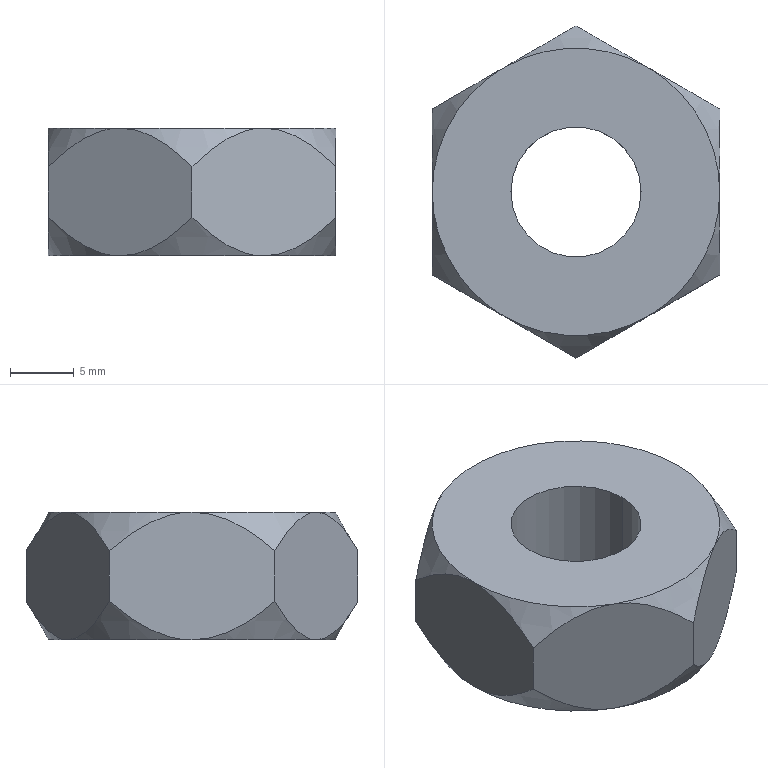Part | SolidWorks | features 3DProfileFeature 1, Extrusion 1, HoleWzd 1, ICE 1, MirrorPattern 1 | 1 solid | 22 faces | box 22.517 x 26 x 10 mm | volume 3499 mm3 | cone 12 | plane 8 | cylinder 2 | commonest cylinder face diameters 10.2 x2
STEP:
#1=CARTESIAN_POINT('',(-5.1,0.,-5.));
#2=VERTEX_POINT('',#1);
#3=CARTESIAN_POINT('',(5.1,0.,-5.));
#4=VERTEX_POINT('',#3);
#5=CARTESIAN_POINT('',(0.,0.,-5.));
#6=DIRECTION('',(0.,0.,1.));
#7=DIRECTION('',(1.,0.,0.));
#8=AXIS2_PLACEMENT_3D('',#5,#6,#7);
#9=CIRCLE('',#8,5.1);
#10=EDGE_CURVE('',#2,#4,#9,.T.);
#11=ORIENTED_EDGE('',*,*,#10,.F.);
#12=CARTESIAN_POINT('',(-5.1,0.,5.));
#13=VERTEX_POINT('',#12);
#14=CARTESIAN_POINT('',(-5.1,0.,5.));
#15=DIRECTION('',(0.,0.,1.));
#16=VECTOR('',#15,1000.);
#17=LINE('',#14,#16);
#18=EDGE_CURVE('',#2,#13,#17,.T.);
#19=ORIENTED_EDGE('',*,*,#18,.T.);
#20=CARTESIAN_POINT('',(5.1,0.,5.));
#21=VERTEX_POINT('',#20);
#22=CARTESIAN_POINT('',(0.,0.,5.));
#23=DIRECTION('',(0.,0.,1.));
#24=DIRECTION('',(1.,0.,0.));
#25=AXIS2_PLACEMENT_3D('',#22,#23,#24);
#26=CIRCLE('',#25,5.1);
#27=EDGE_CURVE('',#13,#21,#26,.T.);
#28=ORIENTED_EDGE('',*,*,#27,.T.);
#29=CARTESIAN_POINT('',(5.1,0.,5.));
#30=DIRECTION('',(0.,0.,1.));
#31=VECTOR('',#30,1000.);
#32=LINE('',#29,#31);
#33=EDGE_CURVE('',#4,#21,#32,.T.);
#34=ORIENTED_EDGE('',*,*,#33,.F.);
#35=EDGE_LOOP('',(#11,#19,#28,#34));
#36=FACE_OUTER_BOUND('',#35,.T.);
#37=CARTESIAN_POINT('',(0.,0.,5.));
#38=DIRECTION('',(0.,0.,1.));
#39=DIRECTION('',(1.,0.,0.));
#40=AXIS2_PLACEMENT_3D('',#37,#38,#39);
#41=CYLINDRICAL_SURFACE('',#40,5.1);
#42=ADVANCED_FACE('',(#36),#41,.F.);
#43=CARTESIAN_POINT('',(11.258,6.5,1.983));
#44=VERTEX_POINT('',#43);
#45=CARTESIAN_POINT('',(11.258,6.5,-1.983));
#46=VERTEX_POINT('',#45);
#47=CARTESIAN_POINT('',(11.258,6.5,5.));
#48=DIRECTION('',(0.,0.,-1.));
#49=VECTOR('',#48,1000.);
#50=LINE('',#47,#49);
#51=EDGE_CURVE('',#44,#46,#50,.T.);
#52=ORIENTED_EDGE('',*,*,#51,.T.);
#53=CARTESIAN_POINT('',(5.629,9.75,-5.));
#54=VERTEX_POINT('',#53);
#55=CARTESIAN_POINT('',(11.258,6.5,-1.983));
#56=CARTESIAN_POINT('',(10.858,6.731,-2.384));
#57=CARTESIAN_POINT('',(10.446,6.969,-2.764));
#58=CARTESIAN_POINT('',(9.589,7.464,-3.467));
#59=CARTESIAN_POINT('',(9.145,7.72,-3.79));
#60=CARTESIAN_POINT('',(8.441,8.126,-4.21));
#61=CARTESIAN_POINT('',(8.199,8.266,-4.34));
#62=CARTESIAN_POINT('',(7.705,8.551,-4.569));
#63=CARTESIAN_POINT('',(7.455,8.696,-4.667));
#64=CARTESIAN_POINT('',(6.946,8.99,-4.829));
#65=CARTESIAN_POINT('',(6.688,9.139,-4.892));
#66=CARTESIAN_POINT('',(6.162,9.442,-4.978));
#67=CARTESIAN_POINT('',(5.894,9.597,-5.));
#68=CARTESIAN_POINT('',(5.629,9.75,-5.));
#69=B_SPLINE_CURVE_WITH_KNOTS('',3,(#55,#56,#57,#58,#59,#60,#61,#62,#63,#64,#65,#66,#67,#68),.UNSPECIFIED.,.F.,.F.,(4,2,2,2,2,2,4),(0.000000303,0.001819,0.003638,0.004548,0.005458,0.006367,0.007277),.UNSPECIFIED.);
#70=EDGE_CURVE('',#46,#54,#69,.T.);
#71=ORIENTED_EDGE('',*,*,#70,.T.);
#72=CARTESIAN_POINT('',(0.,13.,-1.983));
#73=VERTEX_POINT('',#72);
#74=CARTESIAN_POINT('',(5.629,9.75,-5.));
#75=CARTESIAN_POINT('',(5.101,10.055,-5.));
#76=CARTESIAN_POINT('',(4.58,10.356,-4.914));
#77=CARTESIAN_POINT('',(3.553,10.949,-4.589));
#78=CARTESIAN_POINT('',(3.064,11.231,-4.356));
#79=CARTESIAN_POINT('',(2.129,11.771,-3.801));
#80=CARTESIAN_POINT('',(1.679,12.031,-3.475));
#81=CARTESIAN_POINT('',(0.8147,12.53,-2.766));
#82=CARTESIAN_POINT('',(0.401,12.768,-2.384));
#83=CARTESIAN_POINT('',(0.,13.,-1.983));
#84=B_SPLINE_CURVE_WITH_KNOTS('',3,(#74,#75,#76,#77,#78,#79,#80,#81,#82,#83),.UNSPECIFIED.,.F.,.F.,(4,2,2,2,4),(0.007277,0.009093,0.01091,0.01272,0.01454),.UNSPECIFIED.);
#85=EDGE_CURVE('',#54,#73,#84,.T.);
#86=ORIENTED_EDGE('',*,*,#85,.T.);
#87=CARTESIAN_POINT('',(0.,13.,1.983));
#88=VERTEX_POINT('',#87);
#89=CARTESIAN_POINT('',(0.,13.,5.));
#90=DIRECTION('',(0.,0.,-1.));
#91=VECTOR('',#90,1000.);
#92=LINE('',#89,#91);
#93=EDGE_CURVE('',#88,#73,#92,.T.);
#94=ORIENTED_EDGE('',*,*,#93,.F.);
#95=CARTESIAN_POINT('',(5.629,9.75,5.));
#96=VERTEX_POINT('',#95);
#97=CARTESIAN_POINT('',(5.629,9.75,5.));
#98=CARTESIAN_POINT('',(5.101,10.055,5.));
#99=CARTESIAN_POINT('',(4.58,10.356,4.914));
#100=CARTESIAN_POINT('',(3.553,10.949,4.589));
#101=CARTESIAN_POINT('',(3.064,11.231,4.356));
#102=CARTESIAN_POINT('',(2.129,11.771,3.801));
#103=CARTESIAN_POINT('',(1.679,12.031,3.475));
#104=CARTESIAN_POINT('',(0.8147,12.53,2.766));
#105=CARTESIAN_POINT('',(0.401,12.768,2.384));
#106=CARTESIAN_POINT('',(0.,13.,1.983));
#107=B_SPLINE_CURVE_WITH_KNOTS('',3,(#97,#98,#99,#100,#101,#102,#103,#104,#105,#106),.UNSPECIFIED.,.F.,.F.,(4,2,2,2,4),(0.007277,0.009093,0.01091,0.01272,0.01454),.UNSPECIFIED.);
#108=EDGE_CURVE('',#96,#88,#107,.T.);
#109=ORIENTED_EDGE('',*,*,#108,.F.);
#110=CARTESIAN_POINT('',(11.258,6.5,1.983));
#111=CARTESIAN_POINT('',(10.858,6.731,2.384));
#112=CARTESIAN_POINT('',(10.446,6.969,2.764));
#113=CARTESIAN_POINT('',(9.589,7.464,3.467));
#114=CARTESIAN_POINT('',(9.145,7.72,3.79));
#115=CARTESIAN_POINT('',(8.441,8.126,4.21));
#116=CARTESIAN_POINT('',(8.199,8.266,4.34));
#117=CARTESIAN_POINT('',(7.705,8.551,4.569));
#118=CARTESIAN_POINT('',(7.455,8.696,4.667));
#119=CARTESIAN_POINT('',(6.946,8.99,4.829));
#120=CARTESIAN_POINT('',(6.688,9.139,4.892));
#121=CARTESIAN_POINT('',(6.162,9.442,4.978));
#122=CARTESIAN_POINT('',(5.894,9.597,5.));
#123=CARTESIAN_POINT('',(5.629,9.75,5.));
#124=B_SPLINE_CURVE_WITH_KNOTS('',3,(#110,#111,#112,#113,#114,#115,#116,#117,#118,#119,#120,#121,#122,#123),.UNSPECIFIED.,.F.,.F.,(4,2,2,2,2,2,4),(0.000000303,0.001819,0.003638,0.004548,0.005458,0.006367,0.007277),.UNSPECIFIED.);
#125=EDGE_CURVE('',#44,#96,#124,.T.);
#126=ORIENTED_EDGE('',*,*,#125,.F.);
#127=EDGE_LOOP('',(#52,#71,#86,#94,#109,#126));
#128=FACE_OUTER_BOUND('',#127,.T.);
#129=CARTESIAN_POINT('',(11.258,6.5,5.));
#130=DIRECTION('',(-0.5,-0.866,0.));
#131=DIRECTION('',(0.866,-0.5,0.));
#132=AXIS2_PLACEMENT_3D('',#129,#130,#131);
#133=PLANE('',#132);
#134=ADVANCED_FACE('',(#128),#133,.F.);
#135=ORIENTED_EDGE('',*,*,#93,.T.);
#136=CARTESIAN_POINT('',(-5.629,9.75,-5.));
#137=VERTEX_POINT('',#136);
#138=CARTESIAN_POINT('',(0.,13.,-1.983));
#139=CARTESIAN_POINT('',(-0.4004,12.769,-2.384));
#140=CARTESIAN_POINT('',(-0.8123,12.531,-2.764));
#141=CARTESIAN_POINT('',(-1.669,12.036,-3.467));
#142=CARTESIAN_POINT('',(-2.113,11.78,-3.79));
#143=CARTESIAN_POINT('',(-2.817,11.374,-4.21));
#144=CARTESIAN_POINT('',(-3.059,11.234,-4.34));
#145=CARTESIAN_POINT('',(-3.553,10.949,-4.569));
#146=CARTESIAN_POINT('',(-3.803,10.804,-4.667));
#147=CARTESIAN_POINT('',(-4.312,10.51,-4.829));
#148=CARTESIAN_POINT('',(-4.57,10.361,-4.892));
#149=CARTESIAN_POINT('',(-5.096,10.058,-4.978));
#150=CARTESIAN_POINT('',(-5.365,9.903,-5.));
#151=CARTESIAN_POINT('',(-5.629,9.75,-5.));
#152=B_SPLINE_CURVE_WITH_KNOTS('',3,(#138,#139,#140,#141,#142,#143,#144,#145,#146,#147,#148,#149,#150,#151),.UNSPECIFIED.,.F.,.F.,(4,2,2,2,2,2,4),(0.000000303,0.001819,0.003638,0.004548,0.005458,0.006367,0.007277),.UNSPECIFIED.);
#153=EDGE_CURVE('',#73,#137,#152,.T.);
#154=ORIENTED_EDGE('',*,*,#153,.T.);
#155=CARTESIAN_POINT('',(-11.258,6.5,-1.983));
#156=VERTEX_POINT('',#155);
#157=CARTESIAN_POINT('',(-5.629,9.75,-5.));
#158=CARTESIAN_POINT('',(-6.157,9.445,-5.));
#159=CARTESIAN_POINT('',(-6.678,9.144,-4.914));
#160=CARTESIAN_POINT('',(-7.706,8.551,-4.589));
#161=CARTESIAN_POINT('',(-8.194,8.269,-4.356));
#162=CARTESIAN_POINT('',(-9.129,7.729,-3.801));
#163=CARTESIAN_POINT('',(-9.579,7.469,-3.475));
#164=CARTESIAN_POINT('',(-10.444,6.97,-2.766));
#165=CARTESIAN_POINT('',(-10.857,6.732,-2.384));
#166=CARTESIAN_POINT('',(-11.258,6.5,-1.983));
#167=B_SPLINE_CURVE_WITH_KNOTS('',3,(#157,#158,#159,#160,#161,#162,#163,#164,#165,#166),.UNSPECIFIED.,.F.,.F.,(4,2,2,2,4),(0.007277,0.009093,0.01091,0.01272,0.01454),.UNSPECIFIED.);
#168=EDGE_CURVE('',#137,#156,#167,.T.);
#169=ORIENTED_EDGE('',*,*,#168,.T.);
#170=CARTESIAN_POINT('',(-11.258,6.5,1.983));
#171=VERTEX_POINT('',#170);
#172=CARTESIAN_POINT('',(-11.258,6.5,5.));
#173=DIRECTION('',(0.,0.,-1.));
#174=VECTOR('',#173,1000.);
#175=LINE('',#172,#174);
#176=EDGE_CURVE('',#171,#156,#175,.T.);
#177=ORIENTED_EDGE('',*,*,#176,.F.);
#178=CARTESIAN_POINT('',(-5.629,9.75,5.));
#179=VERTEX_POINT('',#178);
#180=CARTESIAN_POINT('',(-5.629,9.75,5.));
#181=CARTESIAN_POINT('',(-6.157,9.445,5.));
#182=CARTESIAN_POINT('',(-6.678,9.144,4.914));
#183=CARTESIAN_POINT('',(-7.706,8.551,4.589));
#184=CARTESIAN_POINT('',(-8.194,8.269,4.356));
#185=CARTESIAN_POINT('',(-9.129,7.729,3.801));
#186=CARTESIAN_POINT('',(-9.579,7.469,3.475));
#187=CARTESIAN_POINT('',(-10.444,6.97,2.766));
#188=CARTESIAN_POINT('',(-10.857,6.732,2.384));
#189=CARTESIAN_POINT('',(-11.258,6.5,1.983));
#190=B_SPLINE_CURVE_WITH_KNOTS('',3,(#180,#181,#182,#183,#184,#185,#186,#187,#188,#189),.UNSPECIFIED.,.F.,.F.,(4,2,2,2,4),(0.007277,0.009093,0.01091,0.01272,0.01454),.UNSPECIFIED.);
#191=EDGE_CURVE('',#179,#171,#190,.T.);
#192=ORIENTED_EDGE('',*,*,#191,.F.);
#193=CARTESIAN_POINT('',(0.,13.,1.983));
#194=CARTESIAN_POINT('',(-0.4004,12.769,2.384));
#195=CARTESIAN_POINT('',(-0.8123,12.531,2.764));
#196=CARTESIAN_POINT('',(-1.669,12.036,3.467));
#197=CARTESIAN_POINT('',(-2.113,11.78,3.79));
#198=CARTESIAN_POINT('',(-2.817,11.374,4.21));
#199=CARTESIAN_POINT('',(-3.059,11.234,4.34));
#200=CARTESIAN_POINT('',(-3.553,10.949,4.569));
#201=CARTESIAN_POINT('',(-3.803,10.804,4.667));
#202=CARTESIAN_POINT('',(-4.312,10.51,4.829));
#203=CARTESIAN_POINT('',(-4.57,10.361,4.892));
#204=CARTESIAN_POINT('',(-5.096,10.058,4.978));
#205=CARTESIAN_POINT('',(-5.365,9.903,5.));
#206=CARTESIAN_POINT('',(-5.629,9.75,5.));
#207=B_SPLINE_CURVE_WITH_KNOTS('',3,(#193,#194,#195,#196,#197,#198,#199,#200,#201,#202,#203,#204,#205,#206),.UNSPECIFIED.,.F.,.F.,(4,2,2,2,2,2,4),(0.000000303,0.001819,0.003638,0.004548,0.005458,0.006367,0.007277),.UNSPECIFIED.);
#208=EDGE_CURVE('',#88,#179,#207,.T.);
#209=ORIENTED_EDGE('',*,*,#208,.F.);
#210=EDGE_LOOP('',(#135,#154,#169,#177,#192,#209));
#211=FACE_OUTER_BOUND('',#210,.T.);
#212=CARTESIAN_POINT('',(0.,13.,5.));
#213=DIRECTION('',(0.5,-0.866,0.));
#214=DIRECTION('',(0.866,0.5,0.));
#215=AXIS2_PLACEMENT_3D('',#212,#213,#214);
#216=PLANE('',#215);
#217=ADVANCED_FACE('',(#211),#216,.F.);
#218=ORIENTED_EDGE('',*,*,#176,.T.);
#219=CARTESIAN_POINT('',(-11.258,0.,-5.));
#220=VERTEX_POINT('',#219);
#221=CARTESIAN_POINT('',(-11.258,6.5,-1.983));
#222=CARTESIAN_POINT('',(-11.258,6.271,-2.182));
#223=CARTESIAN_POINT('',(-11.258,6.038,-2.376));
#224=CARTESIAN_POINT('',(-11.258,5.56,-2.755));
#225=CARTESIAN_POINT('',(-11.258,5.315,-2.94));
#226=CARTESIAN_POINT('',(-11.258,4.568,-3.471));
#227=CARTESIAN_POINT('',(-11.258,4.053,-3.794));
#228=CARTESIAN_POINT('',(-11.258,3.243,-4.212));
#229=CARTESIAN_POINT('',(-11.258,2.966,-4.34));
#230=CARTESIAN_POINT('',(-11.258,2.398,-4.568));
#231=CARTESIAN_POINT('',(-11.258,2.105,-4.668));
#232=CARTESIAN_POINT('',(-11.258,1.516,-4.83));
#233=CARTESIAN_POINT('',(-11.258,1.218,-4.893));
#234=CARTESIAN_POINT('',(-11.258,0.6148,-4.978));
#235=CARTESIAN_POINT('',(-11.258,0.3082,-5.));
#236=CARTESIAN_POINT('',(-11.258,0.,-5.));
#237=B_SPLINE_CURVE_WITH_KNOTS('',3,(#221,#222,#223,#224,#225,#226,#227,#228,#229,#230,#231,#232,#233,#234,#235,#236),.UNSPECIFIED.,.F.,.F.,(4,2,2,2,2,2,2,4),(0.01214,0.01304,0.01394,0.01574,0.01665,0.01755,0.01845,0.01935),.UNSPECIFIED.);
#238=EDGE_CURVE('',#156,#220,#237,.T.);
#239=ORIENTED_EDGE('',*,*,#238,.T.);
#240=CARTESIAN_POINT('',(-11.258,-6.5,-1.983));
#241=VERTEX_POINT('',#240);
#242=CARTESIAN_POINT('',(-11.258,0.,-5.));
#243=CARTESIAN_POINT('',(-11.258,-0.6167,-5.));
#244=CARTESIAN_POINT('',(-11.258,-1.219,-4.912));
#245=CARTESIAN_POINT('',(-11.258,-2.105,-4.668));
#246=CARTESIAN_POINT('',(-11.258,-2.398,-4.568));
#247=CARTESIAN_POINT('',(-11.258,-2.966,-4.341));
#248=CARTESIAN_POINT('',(-11.258,-3.242,-4.213));
#249=CARTESIAN_POINT('',(-11.258,-4.052,-3.795));
#250=CARTESIAN_POINT('',(-11.258,-4.567,-3.471));
#251=CARTESIAN_POINT('',(-11.258,-5.565,-2.762));
#252=CARTESIAN_POINT('',(-11.258,-6.042,-2.38));
#253=CARTESIAN_POINT('',(-11.258,-6.5,-1.983));
#254=B_SPLINE_CURVE_WITH_KNOTS('',3,(#242,#243,#244,#245,#246,#247,#248,#249,#250,#251,#252,#253),.UNSPECIFIED.,.F.,.F.,(4,2,2,2,2,4),(0.01935,0.02115,0.02206,0.02296,0.02476,0.02656),.UNSPECIFIED.);
#255=EDGE_CURVE('',#220,#241,#254,.T.);
#256=ORIENTED_EDGE('',*,*,#255,.T.);
#257=CARTESIAN_POINT('',(-11.258,-6.5,1.983));
#258=VERTEX_POINT('',#257);
#259=CARTESIAN_POINT('',(-11.258,-6.5,5.));
#260=DIRECTION('',(0.,0.,-1.));
#261=VECTOR('',#260,1000.);
#262=LINE('',#259,#261);
#263=EDGE_CURVE('',#258,#241,#262,.T.);
#264=ORIENTED_EDGE('',*,*,#263,.F.);
#265=CARTESIAN_POINT('',(-11.258,0.,5.));
#266=VERTEX_POINT('',#265);
#267=CARTESIAN_POINT('',(-11.258,0.,5.));
#268=CARTESIAN_POINT('',(-11.258,-0.6167,5.));
#269=CARTESIAN_POINT('',(-11.258,-1.219,4.912));
#270=CARTESIAN_POINT('',(-11.258,-2.105,4.668));
#271=CARTESIAN_POINT('',(-11.258,-2.398,4.568));
#272=CARTESIAN_POINT('',(-11.258,-2.966,4.341));
#273=CARTESIAN_POINT('',(-11.258,-3.242,4.213));
#274=CARTESIAN_POINT('',(-11.258,-4.052,3.795));
#275=CARTESIAN_POINT('',(-11.258,-4.567,3.471));
#276=CARTESIAN_POINT('',(-11.258,-5.565,2.762));
#277=CARTESIAN_POINT('',(-11.258,-6.042,2.38));
#278=CARTESIAN_POINT('',(-11.258,-6.5,1.983));
#279=B_SPLINE_CURVE_WITH_KNOTS('',3,(#267,#268,#269,#270,#271,#272,#273,#274,#275,#276,#277,#278),.UNSPECIFIED.,.F.,.F.,(4,2,2,2,2,4),(0.01935,0.02115,0.02206,0.02296,0.02476,0.02656),.UNSPECIFIED.);
#280=EDGE_CURVE('',#266,#258,#279,.T.);
#281=ORIENTED_EDGE('',*,*,#280,.F.);
#282=CARTESIAN_POINT('',(-11.258,6.5,1.983));
#283=CARTESIAN_POINT('',(-11.258,6.271,2.182));
#284=CARTESIAN_POINT('',(-11.258,6.038,2.376));
#285=CARTESIAN_POINT('',(-11.258,5.56,2.755));
#286=CARTESIAN_POINT('',(-11.258,5.315,2.94));
#287=CARTESIAN_POINT('',(-11.258,4.568,3.471));
#288=CARTESIAN_POINT('',(-11.258,4.053,3.794));
#289=CARTESIAN_POINT('',(-11.258,3.243,4.212));
#290=CARTESIAN_POINT('',(-11.258,2.966,4.34));
#291=CARTESIAN_POINT('',(-11.258,2.398,4.568));
#292=CARTESIAN_POINT('',(-11.258,2.105,4.668));
#293=CARTESIAN_POINT('',(-11.258,1.516,4.83));
#294=CARTESIAN_POINT('',(-11.258,1.218,4.893));
#295=CARTESIAN_POINT('',(-11.258,0.6148,4.978));
#296=CARTESIAN_POINT('',(-11.258,0.3082,5.));
#297=CARTESIAN_POINT('',(-11.258,0.,5.));
#298=B_SPLINE_CURVE_WITH_KNOTS('',3,(#282,#283,#284,#285,#286,#287,#288,#289,#290,#291,#292,#293,#294,#295,#296,#297),.UNSPECIFIED.,.F.,.F.,(4,2,2,2,2,2,2,4),(0.01214,0.01304,0.01394,0.01574,0.01665,0.01755,0.01845,0.01935),.UNSPECIFIED.);
#299=EDGE_CURVE('',#171,#266,#298,.T.);
#300=ORIENTED_EDGE('',*,*,#299,.F.);
#301=EDGE_LOOP('',(#218,#239,#256,#264,#281,#300));
#302=FACE_OUTER_BOUND('',#301,.T.);
#303=CARTESIAN_POINT('',(-11.258,6.5,5.));
#304=DIRECTION('',(1.,0.,0.));
#305=DIRECTION('',(0.,0.,-1.));
#306=AXIS2_PLACEMENT_3D('',#303,#304,#305);
#307=PLANE('',#306);
#308=ADVANCED_FACE('',(#302),#307,.F.);
#309=ORIENTED_EDGE('',*,*,#263,.T.);
#310=CARTESIAN_POINT('',(-5.629,-9.75,-5.));
#311=VERTEX_POINT('',#310);
#312=CARTESIAN_POINT('',(-11.258,-6.5,-1.983));
#313=CARTESIAN_POINT('',(-10.858,-6.731,-2.384));
#314=CARTESIAN_POINT('',(-10.446,-6.969,-2.764));
#315=CARTESIAN_POINT('',(-9.589,-7.464,-3.467));
#316=CARTESIAN_POINT('',(-9.145,-7.72,-3.79));
#317=CARTESIAN_POINT('',(-8.441,-8.126,-4.21));
#318=CARTESIAN_POINT('',(-8.199,-8.266,-4.34));
#319=CARTESIAN_POINT('',(-7.705,-8.551,-4.569));
#320=CARTESIAN_POINT('',(-7.455,-8.696,-4.667));
#321=CARTESIAN_POINT('',(-6.946,-8.99,-4.829));
#322=CARTESIAN_POINT('',(-6.688,-9.139,-4.892));
#323=CARTESIAN_POINT('',(-6.162,-9.442,-4.978));
#324=CARTESIAN_POINT('',(-5.894,-9.597,-5.));
#325=CARTESIAN_POINT('',(-5.629,-9.75,-5.));
#326=B_SPLINE_CURVE_WITH_KNOTS('',3,(#312,#313,#314,#315,#316,#317,#318,#319,#320,#321,#322,#323,#324,#325),.UNSPECIFIED.,.F.,.F.,(4,2,2,2,2,2,4),(0.000000303,0.001819,0.003638,0.004548,0.005458,0.006367,0.007277),.UNSPECIFIED.);
#327=EDGE_CURVE('',#241,#311,#326,.T.);
#328=ORIENTED_EDGE('',*,*,#327,.T.);
#329=CARTESIAN_POINT('',(0.,-13.,-1.983));
#330=VERTEX_POINT('',#329);
#331=CARTESIAN_POINT('',(-5.629,-9.75,-5.));
#332=CARTESIAN_POINT('',(-5.101,-10.055,-5.));
#333=CARTESIAN_POINT('',(-4.58,-10.356,-4.914));
#334=CARTESIAN_POINT('',(-3.553,-10.949,-4.589));
#335=CARTESIAN_POINT('',(-3.064,-11.231,-4.356));
#336=CARTESIAN_POINT('',(-2.129,-11.771,-3.801));
#337=CARTESIAN_POINT('',(-1.679,-12.031,-3.475));
#338=CARTESIAN_POINT('',(-0.8147,-12.53,-2.766));
#339=CARTESIAN_POINT('',(-0.401,-12.768,-2.384));
#340=CARTESIAN_POINT('',(0.,-13.,-1.983));
#341=B_SPLINE_CURVE_WITH_KNOTS('',3,(#331,#332,#333,#334,#335,#336,#337,#338,#339,#340),.UNSPECIFIED.,.F.,.F.,(4,2,2,2,4),(0.007277,0.009093,0.01091,0.01272,0.01454),.UNSPECIFIED.);
#342=EDGE_CURVE('',#311,#330,#341,.T.);
#343=ORIENTED_EDGE('',*,*,#342,.T.);
#344=CARTESIAN_POINT('',(0.,-13.,1.983));
#345=VERTEX_POINT('',#344);
#346=CARTESIAN_POINT('',(0.,-13.,5.));
#347=DIRECTION('',(0.,0.,-1.));
#348=VECTOR('',#347,1000.);
#349=LINE('',#346,#348);
#350=EDGE_CURVE('',#345,#330,#349,.T.);
#351=ORIENTED_EDGE('',*,*,#350,.F.);
#352=CARTESIAN_POINT('',(-5.629,-9.75,5.));
#353=VERTEX_POINT('',#352);
#354=CARTESIAN_POINT('',(-5.629,-9.75,5.));
#355=CARTESIAN_POINT('',(-5.101,-10.055,5.));
#356=CARTESIAN_POINT('',(-4.58,-10.356,4.914));
#357=CARTESIAN_POINT('',(-3.553,-10.949,4.589));
#358=CARTESIAN_POINT('',(-3.064,-11.231,4.356));
#359=CARTESIAN_POINT('',(-2.129,-11.771,3.801));
#360=CARTESIAN_POINT('',(-1.679,-12.031,3.475));
#361=CARTESIAN_POINT('',(-0.8147,-12.53,2.766));
#362=CARTESIAN_POINT('',(-0.401,-12.768,2.384));
#363=CARTESIAN_POINT('',(0.,-13.,1.983));
#364=B_SPLINE_CURVE_WITH_KNOTS('',3,(#354,#355,#356,#357,#358,#359,#360,#361,#362,#363),.UNSPECIFIED.,.F.,.F.,(4,2,2,2,4),(0.007277,0.009093,0.01091,0.01272,0.01454),.UNSPECIFIED.);
#365=EDGE_CURVE('',#353,#345,#364,.T.);
#366=ORIENTED_EDGE('',*,*,#365,.F.);
#367=CARTESIAN_POINT('',(-11.258,-6.5,1.983));
#368=CARTESIAN_POINT('',(-10.858,-6.731,2.384));
#369=CARTESIAN_POINT('',(-10.446,-6.969,2.764));
#370=CARTESIAN_POINT('',(-9.589,-7.464,3.467));
#371=CARTESIAN_POINT('',(-9.145,-7.72,3.79));
#372=CARTESIAN_POINT('',(-8.441,-8.126,4.21));
#373=CARTESIAN_POINT('',(-8.199,-8.266,4.34));
#374=CARTESIAN_POINT('',(-7.705,-8.551,4.569));
#375=CARTESIAN_POINT('',(-7.455,-8.696,4.667));
#376=CARTESIAN_POINT('',(-6.946,-8.99,4.829));
#377=CARTESIAN_POINT('',(-6.688,-9.139,4.892));
#378=CARTESIAN_POINT('',(-6.162,-9.442,4.978));
#379=CARTESIAN_POINT('',(-5.894,-9.597,5.));
#380=CARTESIAN_POINT('',(-5.629,-9.75,5.));
#381=B_SPLINE_CURVE_WITH_KNOTS('',3,(#367,#368,#369,#370,#371,#372,#373,#374,#375,#376,#377,#378,#379,#380),.UNSPECIFIED.,.F.,.F.,(4,2,2,2,2,2,4),(0.000000303,0.001819,0.003638,0.004548,0.005458,0.006367,0.007277),.UNSPECIFIED.);
#382=EDGE_CURVE('',#258,#353,#381,.T.);
#383=ORIENTED_EDGE('',*,*,#382,.F.);
#384=EDGE_LOOP('',(#309,#328,#343,#351,#366,#383));
#385=FACE_OUTER_BOUND('',#384,.T.);
#386=CARTESIAN_POINT('',(-11.258,-6.5,5.));
#387=DIRECTION('',(0.5,0.866,0.));
#388=DIRECTION('',(-0.866,0.5,0.));
#389=AXIS2_PLACEMENT_3D('',#386,#387,#388);
#390=PLANE('',#389);
#391=ADVANCED_FACE('',(#385),#390,.F.);
#392=ORIENTED_EDGE('',*,*,#350,.T.);
#393=CARTESIAN_POINT('',(5.629,-9.75,-5.));
#394=VERTEX_POINT('',#393);
#395=CARTESIAN_POINT('',(0.,-13.,-1.983));
#396=CARTESIAN_POINT('',(0.4004,-12.769,-2.384));
#397=CARTESIAN_POINT('',(0.8123,-12.531,-2.764));
#398=CARTESIAN_POINT('',(1.669,-12.036,-3.467));
#399=CARTESIAN_POINT('',(2.113,-11.78,-3.79));
#400=CARTESIAN_POINT('',(2.817,-11.374,-4.21));
#401=CARTESIAN_POINT('',(3.059,-11.234,-4.34));
#402=CARTESIAN_POINT('',(3.553,-10.949,-4.569));
#403=CARTESIAN_POINT('',(3.803,-10.804,-4.667));
#404=CARTESIAN_POINT('',(4.312,-10.51,-4.829));
#405=CARTESIAN_POINT('',(4.57,-10.361,-4.892));
#406=CARTESIAN_POINT('',(5.096,-10.058,-4.978));
#407=CARTESIAN_POINT('',(5.365,-9.903,-5.));
#408=CARTESIAN_POINT('',(5.629,-9.75,-5.));
#409=B_SPLINE_CURVE_WITH_KNOTS('',3,(#395,#396,#397,#398,#399,#400,#401,#402,#403,#404,#405,#406,#407,#408),.UNSPECIFIED.,.F.,.F.,(4,2,2,2,2,2,4),(0.000000303,0.001819,0.003638,0.004548,0.005458,0.006367,0.007277),.UNSPECIFIED.);
#410=EDGE_CURVE('',#330,#394,#409,.T.);
#411=ORIENTED_EDGE('',*,*,#410,.T.);
#412=CARTESIAN_POINT('',(11.258,-6.5,-1.983));
#413=VERTEX_POINT('',#412);
#414=CARTESIAN_POINT('',(5.629,-9.75,-5.));
#415=CARTESIAN_POINT('',(6.157,-9.445,-5.));
#416=CARTESIAN_POINT('',(6.678,-9.144,-4.914));
#417=CARTESIAN_POINT('',(7.706,-8.551,-4.589));
#418=CARTESIAN_POINT('',(8.194,-8.269,-4.356));
#419=CARTESIAN_POINT('',(9.129,-7.729,-3.801));
#420=CARTESIAN_POINT('',(9.579,-7.469,-3.475));
#421=CARTESIAN_POINT('',(10.444,-6.97,-2.766));
#422=CARTESIAN_POINT('',(10.857,-6.732,-2.384));
#423=CARTESIAN_POINT('',(11.258,-6.5,-1.983));
#424=B_SPLINE_CURVE_WITH_KNOTS('',3,(#414,#415,#416,#417,#418,#419,#420,#421,#422,#423),.UNSPECIFIED.,.F.,.F.,(4,2,2,2,4),(0.007277,0.009093,0.01091,0.01272,0.01454),.UNSPECIFIED.);
#425=EDGE_CURVE('',#394,#413,#424,.T.);
#426=ORIENTED_EDGE('',*,*,#425,.T.);
#427=CARTESIAN_POINT('',(11.258,-6.5,1.983));
#428=VERTEX_POINT('',#427);
#429=CARTESIAN_POINT('',(11.258,-6.5,5.));
#430=DIRECTION('',(0.,0.,-1.));
#431=VECTOR('',#430,1000.);
#432=LINE('',#429,#431);
#433=EDGE_CURVE('',#428,#413,#432,.T.);
#434=ORIENTED_EDGE('',*,*,#433,.F.);
#435=CARTESIAN_POINT('',(5.629,-9.75,5.));
#436=VERTEX_POINT('',#435);
#437=CARTESIAN_POINT('',(5.629,-9.75,5.));
#438=CARTESIAN_POINT('',(6.157,-9.445,5.));
#439=CARTESIAN_POINT('',(6.678,-9.144,4.914));
#440=CARTESIAN_POINT('',(7.706,-8.551,4.589));
#441=CARTESIAN_POINT('',(8.194,-8.269,4.356));
#442=CARTESIAN_POINT('',(9.129,-7.729,3.801));
#443=CARTESIAN_POINT('',(9.579,-7.469,3.475));
#444=CARTESIAN_POINT('',(10.444,-6.97,2.766));
#445=CARTESIAN_POINT('',(10.857,-6.732,2.384));
#446=CARTESIAN_POINT('',(11.258,-6.5,1.983));
#447=B_SPLINE_CURVE_WITH_KNOTS('',3,(#437,#438,#439,#440,#441,#442,#443,#444,#445,#446),.UNSPECIFIED.,.F.,.F.,(4,2,2,2,4),(0.007277,0.009093,0.01091,0.01272,0.01454),.UNSPECIFIED.);
#448=EDGE_CURVE('',#436,#428,#447,.T.);
#449=ORIENTED_EDGE('',*,*,#448,.F.);
#450=CARTESIAN_POINT('',(0.,-13.,1.983));
#451=CARTESIAN_POINT('',(0.4004,-12.769,2.384));
#452=CARTESIAN_POINT('',(0.8123,-12.531,2.764));
#453=CARTESIAN_POINT('',(1.669,-12.036,3.467));
#454=CARTESIAN_POINT('',(2.113,-11.78,3.79));
#455=CARTESIAN_POINT('',(2.817,-11.374,4.21));
#456=CARTESIAN_POINT('',(3.059,-11.234,4.34));
#457=CARTESIAN_POINT('',(3.553,-10.949,4.569));
#458=CARTESIAN_POINT('',(3.803,-10.804,4.667));
#459=CARTESIAN_POINT('',(4.312,-10.51,4.829));
#460=CARTESIAN_POINT('',(4.57,-10.361,4.892));
#461=CARTESIAN_POINT('',(5.096,-10.058,4.978));
#462=CARTESIAN_POINT('',(5.365,-9.903,5.));
#463=CARTESIAN_POINT('',(5.629,-9.75,5.));
#464=B_SPLINE_CURVE_WITH_KNOTS('',3,(#450,#451,#452,#453,#454,#455,#456,#457,#458,#459,#460,#461,#462,#463),.UNSPECIFIED.,.F.,.F.,(4,2,2,2,2,2,4),(0.000000303,0.001819,0.003638,0.004548,0.005458,0.006367,0.007277),.UNSPECIFIED.);
#465=EDGE_CURVE('',#345,#436,#464,.T.);
#466=ORIENTED_EDGE('',*,*,#465,.F.);
#467=EDGE_LOOP('',(#392,#411,#426,#434,#449,#466));
#468=FACE_OUTER_BOUND('',#467,.T.);
#469=CARTESIAN_POINT('',(0.,-13.,5.));
#470=DIRECTION('',(-0.5,0.866,0.));
#471=DIRECTION('',(-0.866,-0.5,0.));
#472=AXIS2_PLACEMENT_3D('',#469,#470,#471);
#473=PLANE('',#472);
#474=ADVANCED_FACE('',(#468),#473,.F.);
#475=ORIENTED_EDGE('',*,*,#433,.T.);
#476=CARTESIAN_POINT('',(11.258,0.,-5.));
#477=VERTEX_POINT('',#476);
#478=CARTESIAN_POINT('',(11.258,-6.5,-1.983));
#479=CARTESIAN_POINT('',(11.258,-6.042,-2.38));
#480=CARTESIAN_POINT('',(11.258,-5.565,-2.762));
#481=CARTESIAN_POINT('',(11.258,-4.567,-3.471));
#482=CARTESIAN_POINT('',(11.258,-4.052,-3.795));
#483=CARTESIAN_POINT('',(11.258,-3.242,-4.213));
#484=CARTESIAN_POINT('',(11.258,-2.966,-4.341));
#485=CARTESIAN_POINT('',(11.258,-2.398,-4.568));
#486=CARTESIAN_POINT('',(11.258,-2.105,-4.668));
#487=CARTESIAN_POINT('',(11.258,-1.219,-4.912));
#488=CARTESIAN_POINT('',(11.258,-0.6167,-5.));
#489=CARTESIAN_POINT('',(11.258,0.,-5.));
#490=B_SPLINE_CURVE_WITH_KNOTS('',3,(#478,#479,#480,#481,#482,#483,#484,#485,#486,#487,#488,#489),.UNSPECIFIED.,.F.,.F.,(4,2,2,2,2,4),(0.00934,0.01115,0.01296,0.01386,0.01477,0.01657),.UNSPECIFIED.);
#491=EDGE_CURVE('',#413,#477,#490,.T.);
#492=ORIENTED_EDGE('',*,*,#491,.T.);
#493=CARTESIAN_POINT('',(11.258,0.,-5.));
#494=CARTESIAN_POINT('',(11.258,0.3082,-5.));
#495=CARTESIAN_POINT('',(11.258,0.6148,-4.978));
#496=CARTESIAN_POINT('',(11.258,1.218,-4.893));
#497=CARTESIAN_POINT('',(11.258,1.516,-4.83));
#498=CARTESIAN_POINT('',(11.258,2.105,-4.668));
#499=CARTESIAN_POINT('',(11.258,2.398,-4.568));
#500=CARTESIAN_POINT('',(11.258,2.966,-4.34));
#501=CARTESIAN_POINT('',(11.258,3.243,-4.212));
#502=CARTESIAN_POINT('',(11.258,4.053,-3.794));
#503=CARTESIAN_POINT('',(11.258,4.568,-3.471));
#504=CARTESIAN_POINT('',(11.258,5.315,-2.94));
#505=CARTESIAN_POINT('',(11.258,5.56,-2.755));
#506=CARTESIAN_POINT('',(11.258,6.038,-2.376));
#507=CARTESIAN_POINT('',(11.258,6.271,-2.182));
#508=CARTESIAN_POINT('',(11.258,6.5,-1.983));
#509=B_SPLINE_CURVE_WITH_KNOTS('',3,(#493,#494,#495,#496,#497,#498,#499,#500,#501,#502,#503,#504,#505,#506,#507,#508),.UNSPECIFIED.,.F.,.F.,(4,2,2,2,2,2,2,4),(0.01657,0.01748,0.01838,0.01929,0.02019,0.022,0.0229,0.0238),.UNSPECIFIED.);
#510=EDGE_CURVE('',#477,#46,#509,.T.);
#511=ORIENTED_EDGE('',*,*,#510,.T.);
#512=ORIENTED_EDGE('',*,*,#51,.F.);
#513=CARTESIAN_POINT('',(11.258,0.,5.));
#514=VERTEX_POINT('',#513);
#515=CARTESIAN_POINT('',(11.258,0.,5.));
#516=CARTESIAN_POINT('',(11.258,0.3082,5.));
#517=CARTESIAN_POINT('',(11.258,0.6148,4.978));
#518=CARTESIAN_POINT('',(11.258,1.218,4.893));
#519=CARTESIAN_POINT('',(11.258,1.516,4.83));
#520=CARTESIAN_POINT('',(11.258,2.105,4.668));
#521=CARTESIAN_POINT('',(11.258,2.398,4.568));
#522=CARTESIAN_POINT('',(11.258,2.966,4.34));
#523=CARTESIAN_POINT('',(11.258,3.243,4.212));
#524=CARTESIAN_POINT('',(11.258,4.053,3.794));
#525=CARTESIAN_POINT('',(11.258,4.568,3.471));
#526=CARTESIAN_POINT('',(11.258,5.315,2.94));
#527=CARTESIAN_POINT('',(11.258,5.56,2.755));
#528=CARTESIAN_POINT('',(11.258,6.038,2.376));
#529=CARTESIAN_POINT('',(11.258,6.271,2.182));
#530=CARTESIAN_POINT('',(11.258,6.5,1.983));
#531=B_SPLINE_CURVE_WITH_KNOTS('',3,(#515,#516,#517,#518,#519,#520,#521,#522,#523,#524,#525,#526,#527,#528,#529,#530),.UNSPECIFIED.,.F.,.F.,(4,2,2,2,2,2,2,4),(0.01657,0.01748,0.01838,0.01929,0.02019,0.022,0.0229,0.0238),.UNSPECIFIED.);
#532=EDGE_CURVE('',#514,#44,#531,.T.);
#533=ORIENTED_EDGE('',*,*,#532,.F.);
#534=CARTESIAN_POINT('',(11.258,-6.5,1.983));
#535=CARTESIAN_POINT('',(11.258,-6.042,2.38));
#536=CARTESIAN_POINT('',(11.258,-5.565,2.762));
#537=CARTESIAN_POINT('',(11.258,-4.567,3.471));
#538=CARTESIAN_POINT('',(11.258,-4.052,3.795));
#539=CARTESIAN_POINT('',(11.258,-3.242,4.213));
#540=CARTESIAN_POINT('',(11.258,-2.966,4.341));
#541=CARTESIAN_POINT('',(11.258,-2.398,4.568));
#542=CARTESIAN_POINT('',(11.258,-2.105,4.668));
#543=CARTESIAN_POINT('',(11.258,-1.219,4.912));
#544=CARTESIAN_POINT('',(11.258,-0.6167,5.));
#545=CARTESIAN_POINT('',(11.258,0.,5.));
#546=B_SPLINE_CURVE_WITH_KNOTS('',3,(#534,#535,#536,#537,#538,#539,#540,#541,#542,#543,#544,#545),.UNSPECIFIED.,.F.,.F.,(4,2,2,2,2,4),(0.00934,0.01115,0.01296,0.01386,0.01477,0.01657),.UNSPECIFIED.);
#547=EDGE_CURVE('',#428,#514,#546,.T.);
#548=ORIENTED_EDGE('',*,*,#547,.F.);
#549=EDGE_LOOP('',(#475,#492,#511,#512,#533,#548));
#550=FACE_OUTER_BOUND('',#549,.T.);
#551=CARTESIAN_POINT('',(11.258,-6.5,5.));
#552=DIRECTION('',(-1.,0.,0.));
#553=DIRECTION('',(0.,-1.,0.));
#554=AXIS2_PLACEMENT_3D('',#551,#552,#553);
#555=PLANE('',#554);
#556=ADVANCED_FACE('',(#550),#555,.F.);
#557=ORIENTED_EDGE('',*,*,#448,.T.);
#558=ORIENTED_EDGE('',*,*,#547,.T.);
#559=CARTESIAN_POINT('',(0.,0.,5.));
#560=DIRECTION('',(0.,0.,1.));
#561=DIRECTION('',(1.,0.,0.));
#562=AXIS2_PLACEMENT_3D('',#559,#560,#561);
#563=CIRCLE('',#562,11.258);
#564=EDGE_CURVE('',#436,#514,#563,.T.);
#565=ORIENTED_EDGE('',*,*,#564,.F.);
#566=EDGE_LOOP('',(#557,#558,#565));
#567=FACE_OUTER_BOUND('',#566,.T.);
#568=CARTESIAN_POINT('',(0.,0.,5.));
#569=DIRECTION('',(0.,0.,-1.));
#570=DIRECTION('',(1.,0.,0.));
#571=AXIS2_PLACEMENT_3D('',#568,#569,#570);
#572=CONICAL_SURFACE('',#571,11.258,0.5236);
#573=ADVANCED_FACE('',(#567),#572,.T.);
#574=ORIENTED_EDGE('',*,*,#365,.T.);
#575=ORIENTED_EDGE('',*,*,#465,.T.);
#576=CARTESIAN_POINT('',(0.,0.,5.));
#577=DIRECTION('',(0.,0.,1.));
#578=DIRECTION('',(1.,0.,0.));
#579=AXIS2_PLACEMENT_3D('',#576,#577,#578);
#580=CIRCLE('',#579,11.258);
#581=EDGE_CURVE('',#353,#436,#580,.T.);
#582=ORIENTED_EDGE('',*,*,#581,.F.);
#583=EDGE_LOOP('',(#574,#575,#582));
#584=FACE_OUTER_BOUND('',#583,.T.);
#585=CARTESIAN_POINT('',(0.,0.,5.));
#586=DIRECTION('',(0.,0.,-1.));
#587=DIRECTION('',(1.,0.,0.));
#588=AXIS2_PLACEMENT_3D('',#585,#586,#587);
#589=CONICAL_SURFACE('',#588,11.258,0.5236);
#590=ADVANCED_FACE('',(#584),#589,.T.);
#591=ORIENTED_EDGE('',*,*,#280,.T.);
#592=ORIENTED_EDGE('',*,*,#382,.T.);
#593=CARTESIAN_POINT('',(0.,0.,5.));
#594=DIRECTION('',(0.,0.,1.));
#595=DIRECTION('',(1.,0.,0.));
#596=AXIS2_PLACEMENT_3D('',#593,#594,#595);
#597=CIRCLE('',#596,11.258);
#598=EDGE_CURVE('',#266,#353,#597,.T.);
#599=ORIENTED_EDGE('',*,*,#598,.F.);
#600=EDGE_LOOP('',(#591,#592,#599));
#601=FACE_OUTER_BOUND('',#600,.T.);
#602=CARTESIAN_POINT('',(0.,0.,5.));
#603=DIRECTION('',(0.,0.,-1.));
#604=DIRECTION('',(1.,0.,0.));
#605=AXIS2_PLACEMENT_3D('',#602,#603,#604);
#606=CONICAL_SURFACE('',#605,11.258,0.5236);
#607=ADVANCED_FACE('',(#601),#606,.T.);
#608=ORIENTED_EDGE('',*,*,#191,.T.);
#609=ORIENTED_EDGE('',*,*,#299,.T.);
#610=CARTESIAN_POINT('',(0.,0.,5.));
#611=DIRECTION('',(0.,0.,1.));
#612=DIRECTION('',(1.,0.,0.));
#613=AXIS2_PLACEMENT_3D('',#610,#611,#612);
#614=CIRCLE('',#613,11.258);
#615=EDGE_CURVE('',#179,#266,#614,.T.);
#616=ORIENTED_EDGE('',*,*,#615,.F.);
#617=EDGE_LOOP('',(#608,#609,#616));
#618=FACE_OUTER_BOUND('',#617,.T.);
#619=CARTESIAN_POINT('',(0.,0.,5.));
#620=DIRECTION('',(0.,0.,-1.));
#621=DIRECTION('',(1.,0.,0.));
#622=AXIS2_PLACEMENT_3D('',#619,#620,#621);
#623=CONICAL_SURFACE('',#622,11.258,0.5236);
#624=ADVANCED_FACE('',(#618),#623,.T.);
#625=ORIENTED_EDGE('',*,*,#108,.T.);
#626=ORIENTED_EDGE('',*,*,#208,.T.);
#627=CARTESIAN_POINT('',(0.,0.,5.));
#628=DIRECTION('',(0.,0.,1.));
#629=DIRECTION('',(1.,0.,0.));
#630=AXIS2_PLACEMENT_3D('',#627,#628,#629);
#631=CIRCLE('',#630,11.258);
#632=EDGE_CURVE('',#96,#179,#631,.T.);
#633=ORIENTED_EDGE('',*,*,#632,.F.);
#634=EDGE_LOOP('',(#625,#626,#633));
#635=FACE_OUTER_BOUND('',#634,.T.);
#636=CARTESIAN_POINT('',(0.,0.,5.));
#637=DIRECTION('',(0.,0.,-1.));
#638=DIRECTION('',(1.,0.,0.));
#639=AXIS2_PLACEMENT_3D('',#636,#637,#638);
#640=CONICAL_SURFACE('',#639,11.258,0.5236);
#641=ADVANCED_FACE('',(#635),#640,.T.);
#642=ORIENTED_EDGE('',*,*,#125,.T.);
#643=CARTESIAN_POINT('',(0.,0.,5.));
#644=DIRECTION('',(0.,0.,1.));
#645=DIRECTION('',(1.,0.,0.));
#646=AXIS2_PLACEMENT_3D('',#643,#644,#645);
#647=CIRCLE('',#646,11.258);
#648=EDGE_CURVE('',#514,#96,#647,.T.);
#649=ORIENTED_EDGE('',*,*,#648,.F.);
#650=ORIENTED_EDGE('',*,*,#532,.T.);
#651=EDGE_LOOP('',(#642,#649,#650));
#652=FACE_OUTER_BOUND('',#651,.T.);
#653=CARTESIAN_POINT('',(0.,0.,5.));
#654=DIRECTION('',(0.,0.,-1.));
#655=DIRECTION('',(1.,0.,0.));
#656=AXIS2_PLACEMENT_3D('',#653,#654,#655);
#657=CONICAL_SURFACE('',#656,11.258,0.5236);
#658=ADVANCED_FACE('',(#652),#657,.T.);
#659=CARTESIAN_POINT('',(0.,0.,5.));
#660=DIRECTION('',(0.,0.,1.));
#661=DIRECTION('',(1.,0.,0.));
#662=AXIS2_PLACEMENT_3D('',#659,#660,#661);
#663=CIRCLE('',#662,5.1);
#664=EDGE_CURVE('',#21,#13,#663,.T.);
#665=ORIENTED_EDGE('',*,*,#664,.F.);
#666=ORIENTED_EDGE('',*,*,#27,.F.);
#667=EDGE_LOOP('',(#665,#666));
#668=FACE_BOUND('',#667,.T.);
#669=ORIENTED_EDGE('',*,*,#564,.T.);
#670=ORIENTED_EDGE('',*,*,#648,.T.);
#671=ORIENTED_EDGE('',*,*,#632,.T.);
#672=ORIENTED_EDGE('',*,*,#615,.T.);
#673=ORIENTED_EDGE('',*,*,#598,.T.);
#674=ORIENTED_EDGE('',*,*,#581,.T.);
#675=EDGE_LOOP('',(#669,#670,#671,#672,#673,#674));
#676=FACE_OUTER_BOUND('',#675,.T.);
#677=CARTESIAN_POINT('',(0.,0.,5.));
#678=DIRECTION('',(0.,0.,1.));
#679=DIRECTION('',(1.,0.,0.));
#680=AXIS2_PLACEMENT_3D('',#677,#678,#679);
#681=PLANE('',#680);
#682=ADVANCED_FACE('',(#668,#676),#681,.T.);
#683=ORIENTED_EDGE('',*,*,#510,.F.);
#684=CARTESIAN_POINT('',(0.,0.,-5.));
#685=DIRECTION('',(0.,0.,1.));
#686=DIRECTION('',(1.,0.,0.));
#687=AXIS2_PLACEMENT_3D('',#684,#685,#686);
#688=CIRCLE('',#687,11.258);
#689=EDGE_CURVE('',#477,#54,#688,.T.);
#690=ORIENTED_EDGE('',*,*,#689,.T.);
#691=ORIENTED_EDGE('',*,*,#70,.F.);
#692=EDGE_LOOP('',(#683,#690,#691));
#693=FACE_OUTER_BOUND('',#692,.T.);
#694=CARTESIAN_POINT('',(0.,0.,-5.));
#695=DIRECTION('',(0.,0.,1.));
#696=DIRECTION('',(1.,0.,0.));
#697=AXIS2_PLACEMENT_3D('',#694,#695,#696);
#698=CONICAL_SURFACE('',#697,11.258,0.5236);
#699=ADVANCED_FACE('',(#693),#698,.T.);
#700=CARTESIAN_POINT('',(0.,0.,-5.));
#701=DIRECTION('',(0.,0.,-1.));
#702=DIRECTION('',(1.,0.,0.));
#703=AXIS2_PLACEMENT_3D('',#700,#701,#702);
#704=CIRCLE('',#703,11.258);
#705=EDGE_CURVE('',#137,#54,#704,.T.);
#706=ORIENTED_EDGE('',*,*,#705,.F.);
#707=ORIENTED_EDGE('',*,*,#153,.F.);
#708=ORIENTED_EDGE('',*,*,#85,.F.);
#709=EDGE_LOOP('',(#706,#707,#708));
#710=FACE_OUTER_BOUND('',#709,.T.);
#711=CARTESIAN_POINT('',(0.,0.,-5.));
#712=DIRECTION('',(0.,0.,1.));
#713=DIRECTION('',(1.,0.,0.));
#714=AXIS2_PLACEMENT_3D('',#711,#712,#713);
#715=CONICAL_SURFACE('',#714,11.258,0.5236);
#716=ADVANCED_FACE('',(#710),#715,.T.);
#717=CARTESIAN_POINT('',(0.,0.,-5.));
#718=DIRECTION('',(0.,0.,-1.));
#719=DIRECTION('',(1.,0.,0.));
#720=AXIS2_PLACEMENT_3D('',#717,#718,#719);
#721=CIRCLE('',#720,11.258);
#722=EDGE_CURVE('',#220,#137,#721,.T.);
#723=ORIENTED_EDGE('',*,*,#722,.F.);
#724=ORIENTED_EDGE('',*,*,#238,.F.);
#725=ORIENTED_EDGE('',*,*,#168,.F.);
#726=EDGE_LOOP('',(#723,#724,#725));
#727=FACE_OUTER_BOUND('',#726,.T.);
#728=CARTESIAN_POINT('',(0.,0.,-5.));
#729=DIRECTION('',(0.,0.,1.));
#730=DIRECTION('',(1.,0.,0.));
#731=AXIS2_PLACEMENT_3D('',#728,#729,#730);
#732=CONICAL_SURFACE('',#731,11.258,0.5236);
#733=ADVANCED_FACE('',(#727),#732,.T.);
#734=CARTESIAN_POINT('',(0.,0.,-5.));
#735=DIRECTION('',(0.,0.,-1.));
#736=DIRECTION('',(1.,0.,0.));
#737=AXIS2_PLACEMENT_3D('',#734,#735,#736);
#738=CIRCLE('',#737,11.258);
#739=EDGE_CURVE('',#311,#220,#738,.T.);
#740=ORIENTED_EDGE('',*,*,#739,.F.);
#741=ORIENTED_EDGE('',*,*,#327,.F.);
#742=ORIENTED_EDGE('',*,*,#255,.F.);
#743=EDGE_LOOP('',(#740,#741,#742));
#744=FACE_OUTER_BOUND('',#743,.T.);
#745=CARTESIAN_POINT('',(0.,0.,-5.));
#746=DIRECTION('',(0.,0.,1.));
#747=DIRECTION('',(1.,0.,0.));
#748=AXIS2_PLACEMENT_3D('',#745,#746,#747);
#749=CONICAL_SURFACE('',#748,11.258,0.5236);
#750=ADVANCED_FACE('',(#744),#749,.T.);
#751=CARTESIAN_POINT('',(0.,0.,-5.));
#752=DIRECTION('',(0.,0.,-1.));
#753=DIRECTION('',(1.,0.,0.));
#754=AXIS2_PLACEMENT_3D('',#751,#752,#753);
#755=CIRCLE('',#754,11.258);
#756=EDGE_CURVE('',#394,#311,#755,.T.);
#757=ORIENTED_EDGE('',*,*,#756,.F.);
#758=ORIENTED_EDGE('',*,*,#410,.F.);
#759=ORIENTED_EDGE('',*,*,#342,.F.);
#760=EDGE_LOOP('',(#757,#758,#759));
#761=FACE_OUTER_BOUND('',#760,.T.);
#762=CARTESIAN_POINT('',(0.,0.,-5.));
#763=DIRECTION('',(0.,0.,1.));
#764=DIRECTION('',(1.,0.,0.));
#765=AXIS2_PLACEMENT_3D('',#762,#763,#764);
#766=CONICAL_SURFACE('',#765,11.258,0.5236);
#767=ADVANCED_FACE('',(#761),#766,.T.);
#768=CARTESIAN_POINT('',(0.,0.,-5.));
#769=DIRECTION('',(0.,0.,-1.));
#770=DIRECTION('',(1.,0.,0.));
#771=AXIS2_PLACEMENT_3D('',#768,#769,#770);
#772=CIRCLE('',#771,11.258);
#773=EDGE_CURVE('',#477,#394,#772,.T.);
#774=ORIENTED_EDGE('',*,*,#773,.F.);
#775=ORIENTED_EDGE('',*,*,#491,.F.);
#776=ORIENTED_EDGE('',*,*,#425,.F.);
#777=EDGE_LOOP('',(#774,#775,#776));
#778=FACE_OUTER_BOUND('',#777,.T.);
#779=CARTESIAN_POINT('',(0.,0.,-5.));
#780=DIRECTION('',(0.,0.,1.));
#781=DIRECTION('',(1.,0.,0.));
#782=AXIS2_PLACEMENT_3D('',#779,#780,#781);
#783=CONICAL_SURFACE('',#782,11.258,0.5236);
#784=ADVANCED_FACE('',(#778),#783,.T.);
#785=CARTESIAN_POINT('',(0.,0.,-5.));
#786=DIRECTION('',(0.,0.,1.));
#787=DIRECTION('',(1.,0.,0.));
#788=AXIS2_PLACEMENT_3D('',#785,#786,#787);
#789=CIRCLE('',#788,5.1);
#790=EDGE_CURVE('',#4,#2,#789,.T.);
#791=ORIENTED_EDGE('',*,*,#790,.T.);
#792=ORIENTED_EDGE('',*,*,#10,.T.);
#793=EDGE_LOOP('',(#791,#792));
#794=FACE_BOUND('',#793,.T.);
#795=ORIENTED_EDGE('',*,*,#689,.F.);
#796=ORIENTED_EDGE('',*,*,#773,.T.);
#797=ORIENTED_EDGE('',*,*,#756,.T.);
#798=ORIENTED_EDGE('',*,*,#739,.T.);
#799=ORIENTED_EDGE('',*,*,#722,.T.);
#800=ORIENTED_EDGE('',*,*,#705,.T.);
#801=EDGE_LOOP('',(#795,#796,#797,#798,#799,#800));
#802=FACE_OUTER_BOUND('',#801,.T.);
#803=CARTESIAN_POINT('',(0.,0.,-5.));
#804=DIRECTION('',(0.,0.,1.));
#805=DIRECTION('',(1.,0.,0.));
#806=AXIS2_PLACEMENT_3D('',#803,#804,#805);
#807=PLANE('',#806);
#808=ADVANCED_FACE('',(#794,#802),#807,.F.);
#809=ORIENTED_EDGE('',*,*,#18,.F.);
#810=ORIENTED_EDGE('',*,*,#790,.F.);
#811=ORIENTED_EDGE('',*,*,#33,.T.);
#812=ORIENTED_EDGE('',*,*,#664,.T.);
#813=EDGE_LOOP('',(#809,#810,#811,#812));
#814=FACE_OUTER_BOUND('',#813,.T.);
#815=CARTESIAN_POINT('',(0.,0.,5.));
#816=DIRECTION('',(0.,0.,1.));
#817=DIRECTION('',(1.,0.,0.));
#818=AXIS2_PLACEMENT_3D('',#815,#816,#817);
#819=CYLINDRICAL_SURFACE('',#818,5.1);
#820=ADVANCED_FACE('',(#814),#819,.F.);
#821=CLOSED_SHELL('',(#42,#134,#217,#308,#391,#474,#556,#573,#590,#607,#624,#641,#658,#682,#699,#716,#733,#750,#767,#784,#808,#820));
#822=MANIFOLD_SOLID_BREP('',#821);
#823=CARTESIAN_POINT('',(0.,0.,0.));
#824=DIRECTION('',(0.,0.,1.));
#825=DIRECTION('',(1.,0.,0.));
#826=AXIS2_PLACEMENT_3D('',#823,#824,#825);
#827=(LENGTH_UNIT()NAMED_UNIT(*)SI_UNIT(.MILLI.,.METRE.));
#828=UNCERTAINTY_MEASURE_WITH_UNIT(LENGTH_MEASURE(0.00001),#827,'','');
#829=(NAMED_UNIT(*)PLANE_ANGLE_UNIT()SI_UNIT($,.RADIAN.));
#830=(NAMED_UNIT(*)SI_UNIT($,.STERADIAN.)SOLID_ANGLE_UNIT());
#831=(GEOMETRIC_REPRESENTATION_CONTEXT(3)GLOBAL_UNCERTAINTY_ASSIGNED_CONTEXT((#828))GLOBAL_UNIT_ASSIGNED_CONTEXT((#827,#829,#830))REPRESENTATION_CONTEXT('',''));
#832=ADVANCED_BREP_SHAPE_REPRESENTATION('',(#822,#826),#831);